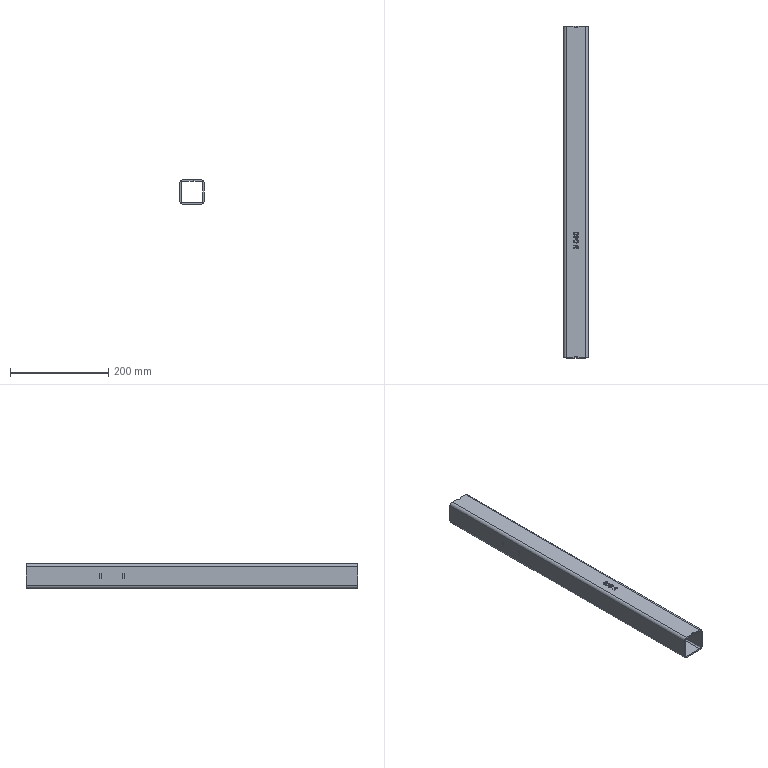Part | SolidWorks | features BaseBody 1 | 1 solid | 87 faces | box 50 x 676 x 50 mm | volume 365028 mm3 | plane 52 | spline 25 | cylinder 10 | commonest cylinder face diameters 6 x4 12 x4 8 x2